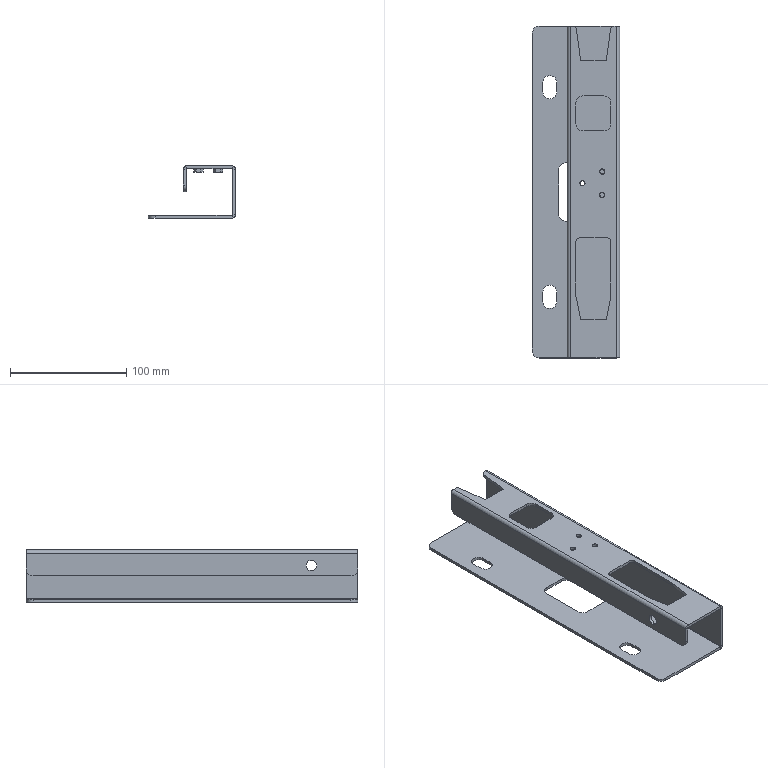Part | SolidWorks | features BaseBody 1 | 1 solid | 112 faces | box 75 x 285 x 45 mm | volume 112519 mm3 | plane 70 | cylinder 42 | commonest cylinder face diameters 12 x16 6 x7 4 x6 4.5 x6 9 x4 1 x3